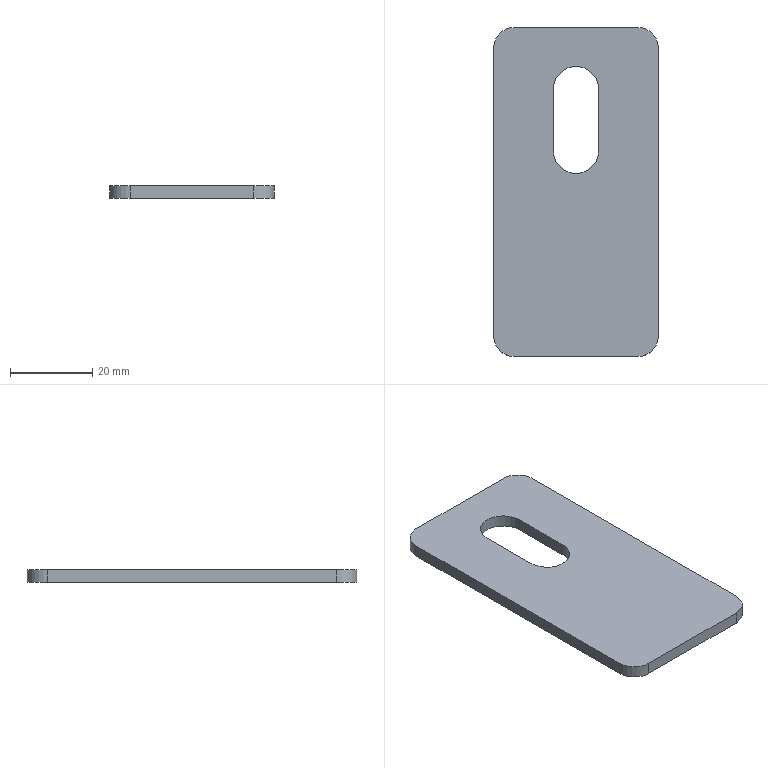Part | STEP file | Part4 | 1 solid | 14 faces | box 40 x 80 x 3 mm | volume 8756 mm3 | plane 8 | cylinder 6 | commonest cylinder face diameters 10 x4 11 x2
STEP:
#1=CARTESIAN_POINT('',(0.,0.,0.));
#2=DIRECTION('',(0.,0.,1.));
#3=DIRECTION('',(1.,0.,0.));
#4=AXIS2_PLACEMENT_3D('',#1,#2,#3);
#5=CARTESIAN_POINT('',(25.5,-30.,0.));
#6=VERTEX_POINT('',#5);
#7=CARTESIAN_POINT('',(25.5,-15.,0.));
#8=VERTEX_POINT('',#7);
#9=CARTESIAN_POINT('',(25.5,-35.,0.));
#10=DIRECTION('',(0.,1.,0.));
#11=VECTOR('',#10,1.);
#12=LINE('',#9,#11);
#13=CARTESIAN_POINT('',(25.5,-30.,0.));
#14=DIRECTION('',(1.,0.,0.));
#15=DIRECTION('',(0.,1.,0.));
#16=AXIS2_PLACEMENT_3D('',#13,#14,#15);
#17=PLANE('',#16);
#18=CARTESIAN_POINT('',(-5.,0.));
#19=DIRECTION('',(1.,0.));
#20=VECTOR('',#19,1.);
#21=LINE('',#18,#20);
#22=(GEOMETRIC_REPRESENTATION_CONTEXT(2)PARAMETRIC_REPRESENTATION_CONTEXT()REPRESENTATION_CONTEXT('',''));
#23=DEFINITIONAL_REPRESENTATION('',(#21),#22);
#24=PCURVE('',#17,#23);
#25=CARTESIAN_POINT('',(20.,-40.,0.));
#26=DIRECTION('',(0.,0.,1.));
#27=DIRECTION('',(1.,0.,0.));
#28=AXIS2_PLACEMENT_3D('',#25,#26,#27);
#29=PLANE('',#28);
#30=CARTESIAN_POINT('',(5.5,5.));
#31=DIRECTION('',(0.,1.));
#32=VECTOR('',#31,1.);
#33=LINE('',#30,#32);
#34=(GEOMETRIC_REPRESENTATION_CONTEXT(2)PARAMETRIC_REPRESENTATION_CONTEXT()REPRESENTATION_CONTEXT('',''));
#35=DEFINITIONAL_REPRESENTATION('',(#33),#34);
#36=PCURVE('',#29,#35);
#37=SURFACE_CURVE('',#12,(#24,#36),.PCURVE_S1.);
#38=EDGE_CURVE('',#6,#8,#37,.T.);
#39=ORIENTED_EDGE('',*,*,#38,.F.);
#40=CARTESIAN_POINT('',(25.5,-30.,3.));
#41=VERTEX_POINT('',#40);
#42=CARTESIAN_POINT('',(25.5,-30.,0.));
#43=DIRECTION('',(0.,0.,-1.));
#44=VECTOR('',#43,1.);
#45=LINE('',#42,#44);
#46=CARTESIAN_POINT('',(0.,0.));
#47=DIRECTION('',(0.,-1.));
#48=VECTOR('',#47,1.);
#49=LINE('',#46,#48);
#50=(GEOMETRIC_REPRESENTATION_CONTEXT(2)PARAMETRIC_REPRESENTATION_CONTEXT()REPRESENTATION_CONTEXT('',''));
#51=DEFINITIONAL_REPRESENTATION('',(#49),#50);
#52=PCURVE('',#17,#51);
#53=CARTESIAN_POINT('',(20.,-30.,0.));
#54=DIRECTION('',(0.,0.,1.));
#55=DIRECTION('',(-1.,0.,0.));
#56=AXIS2_PLACEMENT_3D('',#53,#54,#55);
#57=CYLINDRICAL_SURFACE('',#56,5.5);
#58=CARTESIAN_POINT('',(3.142,0.));
#59=DIRECTION('',(0.,-1.));
#60=VECTOR('',#59,1.);
#61=LINE('',#58,#60);
#62=(GEOMETRIC_REPRESENTATION_CONTEXT(2)PARAMETRIC_REPRESENTATION_CONTEXT()REPRESENTATION_CONTEXT('',''));
#63=DEFINITIONAL_REPRESENTATION('',(#61),#62);
#64=PCURVE('',#57,#63);
#65=SURFACE_CURVE('',#45,(#52,#64),.PCURVE_S1.);
#66=EDGE_CURVE('',#41,#6,#65,.T.);
#67=ORIENTED_EDGE('',*,*,#66,.F.);
#68=CARTESIAN_POINT('',(25.5,-15.,3.));
#69=VERTEX_POINT('',#68);
#70=CARTESIAN_POINT('',(25.5,-35.,3.));
#71=DIRECTION('',(0.,-1.,0.));
#72=VECTOR('',#71,1.);
#73=LINE('',#70,#72);
#74=CARTESIAN_POINT('',(-5.,3.));
#75=DIRECTION('',(-1.,0.));
#76=VECTOR('',#75,1.);
#77=LINE('',#74,#76);
#78=(GEOMETRIC_REPRESENTATION_CONTEXT(2)PARAMETRIC_REPRESENTATION_CONTEXT()REPRESENTATION_CONTEXT('',''));
#79=DEFINITIONAL_REPRESENTATION('',(#77),#78);
#80=PCURVE('',#17,#79);
#81=CARTESIAN_POINT('',(20.,-40.,3.));
#82=DIRECTION('',(0.,0.,1.));
#83=DIRECTION('',(1.,0.,0.));
#84=AXIS2_PLACEMENT_3D('',#81,#82,#83);
#85=PLANE('',#84);
#86=CARTESIAN_POINT('',(5.5,5.));
#87=DIRECTION('',(0.,-1.));
#88=VECTOR('',#87,1.);
#89=LINE('',#86,#88);
#90=(GEOMETRIC_REPRESENTATION_CONTEXT(2)PARAMETRIC_REPRESENTATION_CONTEXT()REPRESENTATION_CONTEXT('',''));
#91=DEFINITIONAL_REPRESENTATION('',(#89),#90);
#92=PCURVE('',#85,#91);
#93=SURFACE_CURVE('',#73,(#80,#92),.PCURVE_S1.);
#94=EDGE_CURVE('',#69,#41,#93,.T.);
#95=ORIENTED_EDGE('',*,*,#94,.F.);
#96=CARTESIAN_POINT('',(25.5,-15.,0.));
#97=DIRECTION('',(0.,0.,-1.));
#98=VECTOR('',#97,1.);
#99=LINE('',#96,#98);
#100=CARTESIAN_POINT('',(15.,0.));
#101=DIRECTION('',(0.,-1.));
#102=VECTOR('',#101,1.);
#103=LINE('',#100,#102);
#104=(GEOMETRIC_REPRESENTATION_CONTEXT(2)PARAMETRIC_REPRESENTATION_CONTEXT()REPRESENTATION_CONTEXT('',''));
#105=DEFINITIONAL_REPRESENTATION('',(#103),#104);
#106=PCURVE('',#17,#105);
#107=CARTESIAN_POINT('',(20.,-15.,0.));
#108=DIRECTION('',(0.,0.,1.));
#109=DIRECTION('',(-1.,0.,0.));
#110=AXIS2_PLACEMENT_3D('',#107,#108,#109);
#111=CYLINDRICAL_SURFACE('',#110,5.5);
#112=CARTESIAN_POINT('',(3.142,0.));
#113=DIRECTION('',(0.,-1.));
#114=VECTOR('',#113,1.);
#115=LINE('',#112,#114);
#116=(GEOMETRIC_REPRESENTATION_CONTEXT(2)PARAMETRIC_REPRESENTATION_CONTEXT()REPRESENTATION_CONTEXT('',''));
#117=DEFINITIONAL_REPRESENTATION('',(#115),#116);
#118=PCURVE('',#111,#117);
#119=SURFACE_CURVE('',#99,(#106,#118),.PCURVE_S1.);
#120=EDGE_CURVE('',#69,#8,#119,.T.);
#121=ORIENTED_EDGE('',*,*,#120,.T.);
#122=EDGE_LOOP('',(#39,#67,#95,#121));
#123=FACE_BOUND('',#122,.T.);
#124=ADVANCED_FACE('',(#123),#17,.F.);
#125=CARTESIAN_POINT('',(14.5,-15.,0.));
#126=VERTEX_POINT('',#125);
#127=CARTESIAN_POINT('',(14.5,-30.,0.));
#128=VERTEX_POINT('',#127);
#129=CARTESIAN_POINT('',(14.5,-27.5,0.));
#130=DIRECTION('',(0.,-1.,0.));
#131=VECTOR('',#130,1.);
#132=LINE('',#129,#131);
#133=CARTESIAN_POINT('',(14.5,-15.,0.));
#134=DIRECTION('',(-1.,0.,0.));
#135=DIRECTION('',(0.,-1.,0.));
#136=AXIS2_PLACEMENT_3D('',#133,#134,#135);
#137=PLANE('',#136);
#138=CARTESIAN_POINT('',(12.5,0.));
#139=DIRECTION('',(1.,0.));
#140=VECTOR('',#139,1.);
#141=LINE('',#138,#140);
#142=(GEOMETRIC_REPRESENTATION_CONTEXT(2)PARAMETRIC_REPRESENTATION_CONTEXT()REPRESENTATION_CONTEXT('',''));
#143=DEFINITIONAL_REPRESENTATION('',(#141),#142);
#144=PCURVE('',#137,#143);
#145=CARTESIAN_POINT('',(-5.5,12.5));
#146=DIRECTION('',(0.,-1.));
#147=VECTOR('',#146,1.);
#148=LINE('',#145,#147);
#149=(GEOMETRIC_REPRESENTATION_CONTEXT(2)PARAMETRIC_REPRESENTATION_CONTEXT()REPRESENTATION_CONTEXT('',''));
#150=DEFINITIONAL_REPRESENTATION('',(#148),#149);
#151=PCURVE('',#29,#150);
#152=SURFACE_CURVE('',#132,(#144,#151),.PCURVE_S1.);
#153=EDGE_CURVE('',#126,#128,#152,.T.);
#154=ORIENTED_EDGE('',*,*,#153,.F.);
#155=CARTESIAN_POINT('',(14.5,-15.,3.));
#156=VERTEX_POINT('',#155);
#157=CARTESIAN_POINT('',(14.5,-15.,0.));
#158=DIRECTION('',(0.,0.,-1.));
#159=VECTOR('',#158,1.);
#160=LINE('',#157,#159);
#161=CARTESIAN_POINT('',(0.,0.));
#162=DIRECTION('',(0.,-1.));
#163=VECTOR('',#162,1.);
#164=LINE('',#161,#163);
#165=(GEOMETRIC_REPRESENTATION_CONTEXT(2)PARAMETRIC_REPRESENTATION_CONTEXT()REPRESENTATION_CONTEXT('',''));
#166=DEFINITIONAL_REPRESENTATION('',(#164),#165);
#167=PCURVE('',#137,#166);
#168=CARTESIAN_POINT('',(6.283,0.));
#169=DIRECTION('',(0.,-1.));
#170=VECTOR('',#169,1.);
#171=LINE('',#168,#170);
#172=(GEOMETRIC_REPRESENTATION_CONTEXT(2)PARAMETRIC_REPRESENTATION_CONTEXT()REPRESENTATION_CONTEXT('',''));
#173=DEFINITIONAL_REPRESENTATION('',(#171),#172);
#174=PCURVE('',#111,#173);
#175=SURFACE_CURVE('',#160,(#167,#174),.PCURVE_S1.);
#176=EDGE_CURVE('',#156,#126,#175,.T.);
#177=ORIENTED_EDGE('',*,*,#176,.F.);
#178=CARTESIAN_POINT('',(14.5,-30.,3.));
#179=VERTEX_POINT('',#178);
#180=CARTESIAN_POINT('',(14.5,-27.5,3.));
#181=DIRECTION('',(0.,1.,0.));
#182=VECTOR('',#181,1.);
#183=LINE('',#180,#182);
#184=CARTESIAN_POINT('',(12.5,3.));
#185=DIRECTION('',(-1.,0.));
#186=VECTOR('',#185,1.);
#187=LINE('',#184,#186);
#188=(GEOMETRIC_REPRESENTATION_CONTEXT(2)PARAMETRIC_REPRESENTATION_CONTEXT()REPRESENTATION_CONTEXT('',''));
#189=DEFINITIONAL_REPRESENTATION('',(#187),#188);
#190=PCURVE('',#137,#189);
#191=CARTESIAN_POINT('',(-5.5,12.5));
#192=DIRECTION('',(0.,1.));
#193=VECTOR('',#192,1.);
#194=LINE('',#191,#193);
#195=(GEOMETRIC_REPRESENTATION_CONTEXT(2)PARAMETRIC_REPRESENTATION_CONTEXT()REPRESENTATION_CONTEXT('',''));
#196=DEFINITIONAL_REPRESENTATION('',(#194),#195);
#197=PCURVE('',#85,#196);
#198=SURFACE_CURVE('',#183,(#190,#197),.PCURVE_S1.);
#199=EDGE_CURVE('',#179,#156,#198,.T.);
#200=ORIENTED_EDGE('',*,*,#199,.F.);
#201=CARTESIAN_POINT('',(14.5,-30.,0.));
#202=DIRECTION('',(0.,0.,1.));
#203=VECTOR('',#202,1.);
#204=LINE('',#201,#203);
#205=CARTESIAN_POINT('',(15.,0.));
#206=DIRECTION('',(0.,1.));
#207=VECTOR('',#206,1.);
#208=LINE('',#205,#207);
#209=(GEOMETRIC_REPRESENTATION_CONTEXT(2)PARAMETRIC_REPRESENTATION_CONTEXT()REPRESENTATION_CONTEXT('',''));
#210=DEFINITIONAL_REPRESENTATION('',(#208),#209);
#211=PCURVE('',#137,#210);
#212=CARTESIAN_POINT('',(0.,0.));
#213=DIRECTION('',(0.,1.));
#214=VECTOR('',#213,1.);
#215=LINE('',#212,#214);
#216=(GEOMETRIC_REPRESENTATION_CONTEXT(2)PARAMETRIC_REPRESENTATION_CONTEXT()REPRESENTATION_CONTEXT('',''));
#217=DEFINITIONAL_REPRESENTATION('',(#215),#216);
#218=PCURVE('',#57,#217);
#219=SURFACE_CURVE('',#204,(#211,#218),.PCURVE_S1.);
#220=EDGE_CURVE('',#128,#179,#219,.T.);
#221=ORIENTED_EDGE('',*,*,#220,.F.);
#222=EDGE_LOOP('',(#154,#177,#200,#221));
#223=FACE_BOUND('',#222,.T.);
#224=ADVANCED_FACE('',(#223),#137,.F.);
#225=CARTESIAN_POINT('',(0.,-5.,0.));
#226=VERTEX_POINT('',#225);
#227=CARTESIAN_POINT('',(0.,-75.,0.));
#228=VERTEX_POINT('',#227);
#229=CARTESIAN_POINT('',(0.,-5.,0.));
#230=DIRECTION('',(0.,-1.,0.));
#231=VECTOR('',#230,1.);
#232=LINE('',#229,#231);
#233=CARTESIAN_POINT('',(-20.,35.));
#234=DIRECTION('',(0.,-1.));
#235=VECTOR('',#234,1.);
#236=LINE('',#233,#235);
#237=(GEOMETRIC_REPRESENTATION_CONTEXT(2)PARAMETRIC_REPRESENTATION_CONTEXT()REPRESENTATION_CONTEXT('',''));
#238=DEFINITIONAL_REPRESENTATION('',(#236),#237);
#239=PCURVE('',#29,#238);
#240=CARTESIAN_POINT('',(0.,-5.,0.));
#241=DIRECTION('',(-1.,0.,0.));
#242=DIRECTION('',(0.,-1.,0.));
#243=AXIS2_PLACEMENT_3D('',#240,#241,#242);
#244=PLANE('',#243);
#245=CARTESIAN_POINT('',(0.,0.));
#246=DIRECTION('',(1.,0.));
#247=VECTOR('',#246,1.);
#248=LINE('',#245,#247);
#249=(GEOMETRIC_REPRESENTATION_CONTEXT(2)PARAMETRIC_REPRESENTATION_CONTEXT()REPRESENTATION_CONTEXT('',''));
#250=DEFINITIONAL_REPRESENTATION('',(#248),#249);
#251=PCURVE('',#244,#250);
#252=SURFACE_CURVE('',#232,(#239,#251),.PCURVE_S1.);
#253=EDGE_CURVE('',#226,#228,#252,.T.);
#254=ORIENTED_EDGE('',*,*,#253,.F.);
#255=CARTESIAN_POINT('',(5.,0.,0.));
#256=VERTEX_POINT('',#255);
#257=CARTESIAN_POINT('',(5.,-5.,0.));
#258=DIRECTION('',(0.,0.,1.));
#259=DIRECTION('',(0.,1.,0.));
#260=AXIS2_PLACEMENT_3D('',#257,#258,#259);
#261=CIRCLE('',#260,5.);
#262=CARTESIAN_POINT('',(-15.,35.));
#263=DIRECTION('',(0.,1.));
#264=AXIS2_PLACEMENT_2D('',#262,#263);
#265=CIRCLE('',#264,5.);
#266=(GEOMETRIC_REPRESENTATION_CONTEXT(2)PARAMETRIC_REPRESENTATION_CONTEXT()REPRESENTATION_CONTEXT('',''));
#267=DEFINITIONAL_REPRESENTATION('',(#265),#266);
#268=PCURVE('',#29,#267);
#269=CARTESIAN_POINT('',(5.,-5.,0.));
#270=DIRECTION('',(0.,0.,1.));
#271=DIRECTION('',(0.,1.,0.));
#272=AXIS2_PLACEMENT_3D('',#269,#270,#271);
#273=CYLINDRICAL_SURFACE('',#272,5.);
#274=CARTESIAN_POINT('',(0.,0.));
#275=DIRECTION('',(1.,0.));
#276=VECTOR('',#275,1.);
#277=LINE('',#274,#276);
#278=(GEOMETRIC_REPRESENTATION_CONTEXT(2)PARAMETRIC_REPRESENTATION_CONTEXT()REPRESENTATION_CONTEXT('',''));
#279=DEFINITIONAL_REPRESENTATION('',(#277),#278);
#280=PCURVE('',#273,#279);
#281=SURFACE_CURVE('',#261,(#268,#280),.PCURVE_S1.);
#282=EDGE_CURVE('',#256,#226,#281,.T.);
#283=ORIENTED_EDGE('',*,*,#282,.F.);
#284=CARTESIAN_POINT('',(35.,0.,0.));
#285=VERTEX_POINT('',#284);
#286=CARTESIAN_POINT('',(35.,0.,0.));
#287=DIRECTION('',(-1.,0.,0.));
#288=VECTOR('',#287,1.);
#289=LINE('',#286,#288);
#290=CARTESIAN_POINT('',(15.,40.));
#291=DIRECTION('',(-1.,0.));
#292=VECTOR('',#291,1.);
#293=LINE('',#290,#292);
#294=(GEOMETRIC_REPRESENTATION_CONTEXT(2)PARAMETRIC_REPRESENTATION_CONTEXT()REPRESENTATION_CONTEXT('',''));
#295=DEFINITIONAL_REPRESENTATION('',(#293),#294);
#296=PCURVE('',#29,#295);
#297=CARTESIAN_POINT('',(35.,0.,0.));
#298=DIRECTION('',(0.,1.,0.));
#299=DIRECTION('',(-1.,0.,0.));
#300=AXIS2_PLACEMENT_3D('',#297,#298,#299);
#301=PLANE('',#300);
#302=CARTESIAN_POINT('',(0.,0.));
#303=DIRECTION('',(1.,0.));
#304=VECTOR('',#303,1.);
#305=LINE('',#302,#304);
#306=(GEOMETRIC_REPRESENTATION_CONTEXT(2)PARAMETRIC_REPRESENTATION_CONTEXT()REPRESENTATION_CONTEXT('',''));
#307=DEFINITIONAL_REPRESENTATION('',(#305),#306);
#308=PCURVE('',#301,#307);
#309=SURFACE_CURVE('',#289,(#296,#308),.PCURVE_S1.);
#310=EDGE_CURVE('',#285,#256,#309,.T.);
#311=ORIENTED_EDGE('',*,*,#310,.F.);
#312=CARTESIAN_POINT('',(40.,-5.,0.));
#313=VERTEX_POINT('',#312);
#314=CARTESIAN_POINT('',(35.,-5.,0.));
#315=DIRECTION('',(0.,0.,1.));
#316=DIRECTION('',(1.,0.,0.));
#317=AXIS2_PLACEMENT_3D('',#314,#315,#316);
#318=CIRCLE('',#317,5.);
#319=CARTESIAN_POINT('',(15.,35.));
#320=DIRECTION('',(1.,0.));
#321=AXIS2_PLACEMENT_2D('',#319,#320);
#322=CIRCLE('',#321,5.);
#323=(GEOMETRIC_REPRESENTATION_CONTEXT(2)PARAMETRIC_REPRESENTATION_CONTEXT()REPRESENTATION_CONTEXT('',''));
#324=DEFINITIONAL_REPRESENTATION('',(#322),#323);
#325=PCURVE('',#29,#324);
#326=CARTESIAN_POINT('',(35.,-5.,0.));
#327=DIRECTION('',(0.,0.,1.));
#328=DIRECTION('',(1.,0.,0.));
#329=AXIS2_PLACEMENT_3D('',#326,#327,#328);
#330=CYLINDRICAL_SURFACE('',#329,5.);
#331=CARTESIAN_POINT('',(0.,0.));
#332=DIRECTION('',(1.,0.));
#333=VECTOR('',#332,1.);
#334=LINE('',#331,#333);
#335=(GEOMETRIC_REPRESENTATION_CONTEXT(2)PARAMETRIC_REPRESENTATION_CONTEXT()REPRESENTATION_CONTEXT('',''));
#336=DEFINITIONAL_REPRESENTATION('',(#334),#335);
#337=PCURVE('',#330,#336);
#338=SURFACE_CURVE('',#318,(#325,#337),.PCURVE_S1.);
#339=EDGE_CURVE('',#313,#285,#338,.T.);
#340=ORIENTED_EDGE('',*,*,#339,.F.);
#341=CARTESIAN_POINT('',(40.,-75.,0.));
#342=VERTEX_POINT('',#341);
#343=CARTESIAN_POINT('',(40.,-75.,0.));
#344=DIRECTION('',(0.,1.,0.));
#345=VECTOR('',#344,1.);
#346=LINE('',#343,#345);
#347=CARTESIAN_POINT('',(20.,-35.));
#348=DIRECTION('',(0.,1.));
#349=VECTOR('',#348,1.);
#350=LINE('',#347,#349);
#351=(GEOMETRIC_REPRESENTATION_CONTEXT(2)PARAMETRIC_REPRESENTATION_CONTEXT()REPRESENTATION_CONTEXT('',''));
#352=DEFINITIONAL_REPRESENTATION('',(#350),#351);
#353=PCURVE('',#29,#352);
#354=CARTESIAN_POINT('',(40.,-75.,0.));
#355=DIRECTION('',(1.,0.,0.));
#356=DIRECTION('',(0.,1.,0.));
#357=AXIS2_PLACEMENT_3D('',#354,#355,#356);
#358=PLANE('',#357);
#359=CARTESIAN_POINT('',(0.,0.));
#360=DIRECTION('',(1.,0.));
#361=VECTOR('',#360,1.);
#362=LINE('',#359,#361);
#363=(GEOMETRIC_REPRESENTATION_CONTEXT(2)PARAMETRIC_REPRESENTATION_CONTEXT()REPRESENTATION_CONTEXT('',''));
#364=DEFINITIONAL_REPRESENTATION('',(#362),#363);
#365=PCURVE('',#358,#364);
#366=SURFACE_CURVE('',#346,(#353,#365),.PCURVE_S1.);
#367=EDGE_CURVE('',#342,#313,#366,.T.);
#368=ORIENTED_EDGE('',*,*,#367,.F.);
#369=CARTESIAN_POINT('',(35.,-80.,0.));
#370=VERTEX_POINT('',#369);
#371=CARTESIAN_POINT('',(35.,-75.,0.));
#372=DIRECTION('',(0.,0.,1.));
#373=DIRECTION('',(0.,-1.,0.));
#374=AXIS2_PLACEMENT_3D('',#371,#372,#373);
#375=CIRCLE('',#374,5.);
#376=CARTESIAN_POINT('',(15.,-35.));
#377=DIRECTION('',(0.,-1.));
#378=AXIS2_PLACEMENT_2D('',#376,#377);
#379=CIRCLE('',#378,5.);
#380=(GEOMETRIC_REPRESENTATION_CONTEXT(2)PARAMETRIC_REPRESENTATION_CONTEXT()REPRESENTATION_CONTEXT('',''));
#381=DEFINITIONAL_REPRESENTATION('',(#379),#380);
#382=PCURVE('',#29,#381);
#383=CARTESIAN_POINT('',(35.,-75.,0.));
#384=DIRECTION('',(0.,0.,1.));
#385=DIRECTION('',(0.,-1.,0.));
#386=AXIS2_PLACEMENT_3D('',#383,#384,#385);
#387=CYLINDRICAL_SURFACE('',#386,5.);
#388=CARTESIAN_POINT('',(0.,0.));
#389=DIRECTION('',(1.,0.));
#390=VECTOR('',#389,1.);
#391=LINE('',#388,#390);
#392=(GEOMETRIC_REPRESENTATION_CONTEXT(2)PARAMETRIC_REPRESENTATION_CONTEXT()REPRESENTATION_CONTEXT('',''));
#393=DEFINITIONAL_REPRESENTATION('',(#391),#392);
#394=PCURVE('',#387,#393);
#395=SURFACE_CURVE('',#375,(#382,#394),.PCURVE_S1.);
#396=EDGE_CURVE('',#370,#342,#395,.T.);
#397=ORIENTED_EDGE('',*,*,#396,.F.);
#398=CARTESIAN_POINT('',(5.,-80.,0.));
#399=VERTEX_POINT('',#398);
#400=CARTESIAN_POINT('',(5.,-80.,0.));
#401=DIRECTION('',(1.,0.,0.));
#402=VECTOR('',#401,1.);
#403=LINE('',#400,#402);
#404=CARTESIAN_POINT('',(-15.,-40.));
#405=DIRECTION('',(1.,0.));
#406=VECTOR('',#405,1.);
#407=LINE('',#404,#406);
#408=(GEOMETRIC_REPRESENTATION_CONTEXT(2)PARAMETRIC_REPRESENTATION_CONTEXT()REPRESENTATION_CONTEXT('',''));
#409=DEFINITIONAL_REPRESENTATION('',(#407),#408);
#410=PCURVE('',#29,#409);
#411=CARTESIAN_POINT('',(5.,-80.,0.));
#412=DIRECTION('',(0.,-1.,0.));
#413=DIRECTION('',(1.,0.,0.));
#414=AXIS2_PLACEMENT_3D('',#411,#412,#413);
#415=PLANE('',#414);
#416=CARTESIAN_POINT('',(0.,0.));
#417=DIRECTION('',(1.,0.));
#418=VECTOR('',#417,1.);
#419=LINE('',#416,#418);
#420=(GEOMETRIC_REPRESENTATION_CONTEXT(2)PARAMETRIC_REPRESENTATION_CONTEXT()REPRESENTATION_CONTEXT('',''));
#421=DEFINITIONAL_REPRESENTATION('',(#419),#420);
#422=PCURVE('',#415,#421);
#423=SURFACE_CURVE('',#403,(#410,#422),.PCURVE_S1.);
#424=EDGE_CURVE('',#399,#370,#423,.T.);
#425=ORIENTED_EDGE('',*,*,#424,.F.);
#426=CARTESIAN_POINT('',(5.,-75.,0.));
#427=DIRECTION('',(0.,0.,1.));
#428=DIRECTION('',(-1.,0.,0.));
#429=AXIS2_PLACEMENT_3D('',#426,#427,#428);
#430=CIRCLE('',#429,5.);
#431=CARTESIAN_POINT('',(-15.,-35.));
#432=DIRECTION('',(-1.,0.));
#433=AXIS2_PLACEMENT_2D('',#431,#432);
#434=CIRCLE('',#433,5.);
#435=(GEOMETRIC_REPRESENTATION_CONTEXT(2)PARAMETRIC_REPRESENTATION_CONTEXT()REPRESENTATION_CONTEXT('',''));
#436=DEFINITIONAL_REPRESENTATION('',(#434),#435);
#437=PCURVE('',#29,#436);
#438=CARTESIAN_POINT('',(5.,-75.,0.));
#439=DIRECTION('',(0.,0.,1.));
#440=DIRECTION('',(-1.,0.,0.));
#441=AXIS2_PLACEMENT_3D('',#438,#439,#440);
#442=CYLINDRICAL_SURFACE('',#441,5.);
#443=CARTESIAN_POINT('',(0.,0.));
#444=DIRECTION('',(1.,0.));
#445=VECTOR('',#444,1.);
#446=LINE('',#443,#445);
#447=(GEOMETRIC_REPRESENTATION_CONTEXT(2)PARAMETRIC_REPRESENTATION_CONTEXT()REPRESENTATION_CONTEXT('',''));
#448=DEFINITIONAL_REPRESENTATION('',(#446),#447);
#449=PCURVE('',#442,#448);
#450=SURFACE_CURVE('',#430,(#437,#449),.PCURVE_S1.);
#451=EDGE_CURVE('',#228,#399,#450,.T.);
#452=ORIENTED_EDGE('',*,*,#451,.F.);
#453=EDGE_LOOP('',(#254,#283,#311,#340,#368,#397,#425,#452));
#454=FACE_BOUND('',#453,.T.);
#455=ORIENTED_EDGE('',*,*,#38,.T.);
#456=CARTESIAN_POINT('',(20.,-15.,0.));
#457=DIRECTION('',(0.,0.,1.));
#458=DIRECTION('',(-1.,0.,0.));
#459=AXIS2_PLACEMENT_3D('',#456,#457,#458);
#460=CIRCLE('',#459,5.5);
#461=CARTESIAN_POINT('',(0.,25.));
#462=DIRECTION('',(-1.,0.));
#463=AXIS2_PLACEMENT_2D('',#461,#462);
#464=CIRCLE('',#463,5.5);
#465=(GEOMETRIC_REPRESENTATION_CONTEXT(2)PARAMETRIC_REPRESENTATION_CONTEXT()REPRESENTATION_CONTEXT('',''));
#466=DEFINITIONAL_REPRESENTATION('',(#464),#465);
#467=PCURVE('',#29,#466);
#468=CARTESIAN_POINT('',(0.,0.));
#469=DIRECTION('',(1.,0.));
#470=VECTOR('',#469,1.);
#471=LINE('',#468,#470);
#472=(GEOMETRIC_REPRESENTATION_CONTEXT(2)PARAMETRIC_REPRESENTATION_CONTEXT()REPRESENTATION_CONTEXT('',''));
#473=DEFINITIONAL_REPRESENTATION('',(#471),#472);
#474=PCURVE('',#111,#473);
#475=SURFACE_CURVE('',#460,(#467,#474),.PCURVE_S1.);
#476=EDGE_CURVE('',#8,#126,#475,.T.);
#477=ORIENTED_EDGE('',*,*,#476,.T.);
#478=ORIENTED_EDGE('',*,*,#153,.T.);
#479=CARTESIAN_POINT('',(20.,-30.,0.));
#480=DIRECTION('',(0.,0.,1.));
#481=DIRECTION('',(-1.,0.,0.));
#482=AXIS2_PLACEMENT_3D('',#479,#480,#481);
#483=CIRCLE('',#482,5.5);
#484=CARTESIAN_POINT('',(0.,10.));
#485=DIRECTION('',(-1.,0.));
#486=AXIS2_PLACEMENT_2D('',#484,#485);
#487=CIRCLE('',#486,5.5);
#488=(GEOMETRIC_REPRESENTATION_CONTEXT(2)PARAMETRIC_REPRESENTATION_CONTEXT()REPRESENTATION_CONTEXT('',''));
#489=DEFINITIONAL_REPRESENTATION('',(#487),#488);
#490=PCURVE('',#29,#489);
#491=CARTESIAN_POINT('',(0.,0.));
#492=DIRECTION('',(1.,0.));
#493=VECTOR('',#492,1.);
#494=LINE('',#491,#493);
#495=(GEOMETRIC_REPRESENTATION_CONTEXT(2)PARAMETRIC_REPRESENTATION_CONTEXT()REPRESENTATION_CONTEXT('',''));
#496=DEFINITIONAL_REPRESENTATION('',(#494),#495);
#497=PCURVE('',#57,#496);
#498=SURFACE_CURVE('',#483,(#490,#497),.PCURVE_S1.);
#499=EDGE_CURVE('',#128,#6,#498,.T.);
#500=ORIENTED_EDGE('',*,*,#499,.T.);
#501=EDGE_LOOP('',(#455,#477,#478,#500));
#502=FACE_BOUND('',#501,.T.);
#503=ADVANCED_FACE('',(#454,#502),#29,.F.);
#504=CARTESIAN_POINT('',(20.,-30.,3.));
#505=DIRECTION('',(0.,0.,-1.));
#506=DIRECTION('',(-1.,0.,0.));
#507=AXIS2_PLACEMENT_3D('',#504,#505,#506);
#508=CIRCLE('',#507,5.5);
#509=CARTESIAN_POINT('',(6.283,3.));
#510=DIRECTION('',(-1.,0.));
#511=VECTOR('',#510,1.);
#512=LINE('',#509,#511);
#513=(GEOMETRIC_REPRESENTATION_CONTEXT(2)PARAMETRIC_REPRESENTATION_CONTEXT()REPRESENTATION_CONTEXT('',''));
#514=DEFINITIONAL_REPRESENTATION('',(#512),#513);
#515=PCURVE('',#57,#514);
#516=CARTESIAN_POINT('',(-5.5,10.));
#517=CARTESIAN_POINT('',(-5.5,19.526));
#518=CARTESIAN_POINT('',(2.75,14.763));
#519=CARTESIAN_POINT('',(11.,10.));
#520=CARTESIAN_POINT('',(2.75,5.237));
#521=CARTESIAN_POINT('',(-5.5,0.4737));
#522=CARTESIAN_POINT('',(-5.5,10.));
#523=(BOUNDED_CURVE()B_SPLINE_CURVE(2,(#516,#517,#518,#519,#520,#521,#522),.UNSPECIFIED.,.T.,.F.)B_SPLINE_CURVE_WITH_KNOTS((1,2,2,2,2,1),(-2.094,0.,2.094,4.189,6.283,8.378),.UNSPECIFIED.)CURVE()GEOMETRIC_REPRESENTATION_ITEM()RATIONAL_B_SPLINE_CURVE((1.,0.5,1.,0.5,1.,0.5,1.))REPRESENTATION_ITEM(''));
#524=(GEOMETRIC_REPRESENTATION_CONTEXT(2)PARAMETRIC_REPRESENTATION_CONTEXT()REPRESENTATION_CONTEXT('',''));
#525=DEFINITIONAL_REPRESENTATION('',(#523),#524);
#526=PCURVE('',#85,#525);
#527=SURFACE_CURVE('',#508,(#515,#526),.PCURVE_S1.);
#528=EDGE_CURVE('',#41,#179,#527,.T.);
#529=ORIENTED_EDGE('',*,*,#528,.T.);
#530=ORIENTED_EDGE('',*,*,#220,.F.);
#531=ORIENTED_EDGE('',*,*,#499,.T.);
#532=ORIENTED_EDGE('',*,*,#66,.F.);
#533=EDGE_LOOP('',(#529,#530,#531,#532));
#534=FACE_BOUND('',#533,.F.);
#535=ADVANCED_FACE('',(#534),#57,.F.);
#536=ORIENTED_EDGE('',*,*,#476,.T.);
#537=ORIENTED_EDGE('',*,*,#176,.F.);
#538=CARTESIAN_POINT('',(20.,-15.,3.));
#539=DIRECTION('',(0.,0.,-1.));
#540=DIRECTION('',(-1.,0.,0.));
#541=AXIS2_PLACEMENT_3D('',#538,#539,#540);
#542=CIRCLE('',#541,5.5);
#543=CARTESIAN_POINT('',(6.283,3.));
#544=DIRECTION('',(-1.,0.));
#545=VECTOR('',#544,1.);
#546=LINE('',#543,#545);
#547=(GEOMETRIC_REPRESENTATION_CONTEXT(2)PARAMETRIC_REPRESENTATION_CONTEXT()REPRESENTATION_CONTEXT('',''));
#548=DEFINITIONAL_REPRESENTATION('',(#546),#547);
#549=PCURVE('',#111,#548);
#550=CARTESIAN_POINT('',(-5.5,25.));
#551=CARTESIAN_POINT('',(-5.5,34.526));
#552=CARTESIAN_POINT('',(2.75,29.763));
#553=CARTESIAN_POINT('',(11.,25.));
#554=CARTESIAN_POINT('',(2.75,20.237));
#555=CARTESIAN_POINT('',(-5.5,15.474));
#556=CARTESIAN_POINT('',(-5.5,25.));
#557=(BOUNDED_CURVE()B_SPLINE_CURVE(2,(#550,#551,#552,#553,#554,#555,#556),.UNSPECIFIED.,.T.,.F.)B_SPLINE_CURVE_WITH_KNOTS((1,2,2,2,2,1),(-2.094,0.,2.094,4.189,6.283,8.378),.UNSPECIFIED.)CURVE()GEOMETRIC_REPRESENTATION_ITEM()RATIONAL_B_SPLINE_CURVE((1.,0.5,1.,0.5,1.,0.5,1.))REPRESENTATION_ITEM(''));
#558=(GEOMETRIC_REPRESENTATION_CONTEXT(2)PARAMETRIC_REPRESENTATION_CONTEXT()REPRESENTATION_CONTEXT('',''));
#559=DEFINITIONAL_REPRESENTATION('',(#557),#558);
#560=PCURVE('',#85,#559);
#561=SURFACE_CURVE('',#542,(#549,#560),.PCURVE_S1.);
#562=EDGE_CURVE('',#156,#69,#561,.T.);
#563=ORIENTED_EDGE('',*,*,#562,.T.);
#564=ORIENTED_EDGE('',*,*,#120,.T.);
#565=EDGE_LOOP('',(#536,#537,#563,#564));
#566=FACE_BOUND('',#565,.F.);
#567=ADVANCED_FACE('',(#566),#111,.F.);
#568=ORIENTED_EDGE('',*,*,#282,.T.);
#569=CARTESIAN_POINT('',(0.,-5.,3.));
#570=VERTEX_POINT('',#569);
#571=CARTESIAN_POINT('',(0.,-5.,0.));
#572=DIRECTION('',(0.,0.,1.));
#573=VECTOR('',#572,1.);
#574=LINE('',#571,#573);
#575=CARTESIAN_POINT('',(1.571,0.));
#576=DIRECTION('',(0.,1.));
#577=VECTOR('',#576,1.);
#578=LINE('',#575,#577);
#579=(GEOMETRIC_REPRESENTATION_CONTEXT(2)PARAMETRIC_REPRESENTATION_CONTEXT()REPRESENTATION_CONTEXT('',''));
#580=DEFINITIONAL_REPRESENTATION('',(#578),#579);
#581=PCURVE('',#273,#580);
#582=CARTESIAN_POINT('',(0.,0.));
#583=DIRECTION('',(0.,1.));
#584=VECTOR('',#583,1.);
#585=LINE('',#582,#584);
#586=(GEOMETRIC_REPRESENTATION_CONTEXT(2)PARAMETRIC_REPRESENTATION_CONTEXT()REPRESENTATION_CONTEXT('',''));
#587=DEFINITIONAL_REPRESENTATION('',(#585),#586);
#588=PCURVE('',#244,#587);
#589=SURFACE_CURVE('',#574,(#581,#588),.PCURVE_S1.);
#590=EDGE_CURVE('',#226,#570,#589,.T.);
#591=ORIENTED_EDGE('',*,*,#590,.T.);
#592=CARTESIAN_POINT('',(5.,0.,3.));
#593=VERTEX_POINT('',#592);
#594=CARTESIAN_POINT('',(5.,-5.,3.));
#595=DIRECTION('',(0.,0.,1.));
#596=DIRECTION('',(0.,1.,0.));
#597=AXIS2_PLACEMENT_3D('',#594,#595,#596);
#598=CIRCLE('',#597,5.);
#599=CARTESIAN_POINT('',(0.,3.));
#600=DIRECTION('',(1.,0.));
#601=VECTOR('',#600,1.);
#602=LINE('',#599,#601);
#603=(GEOMETRIC_REPRESENTATION_CONTEXT(2)PARAMETRIC_REPRESENTATION_CONTEXT()REPRESENTATION_CONTEXT('',''));
#604=DEFINITIONAL_REPRESENTATION('',(#602),#603);
#605=PCURVE('',#273,#604);
#606=CARTESIAN_POINT('',(-15.,35.));
#607=DIRECTION('',(0.,1.));
#608=AXIS2_PLACEMENT_2D('',#606,#607);
#609=CIRCLE('',#608,5.);
#610=(GEOMETRIC_REPRESENTATION_CONTEXT(2)PARAMETRIC_REPRESENTATION_CONTEXT()REPRESENTATION_CONTEXT('',''));
#611=DEFINITIONAL_REPRESENTATION('',(#609),#610);
#612=PCURVE('',#85,#611);
#613=SURFACE_CURVE('',#598,(#605,#612),.PCURVE_S1.);
#614=EDGE_CURVE('',#593,#570,#613,.T.);
#615=ORIENTED_EDGE('',*,*,#614,.F.);
#616=CARTESIAN_POINT('',(5.,0.,0.));
#617=DIRECTION('',(0.,0.,1.));
#618=VECTOR('',#617,1.);
#619=LINE('',#616,#618);
#620=CARTESIAN_POINT('',(0.,0.));
#621=DIRECTION('',(0.,1.));
#622=VECTOR('',#621,1.);
#623=LINE('',#620,#622);
#624=(GEOMETRIC_REPRESENTATION_CONTEXT(2)PARAMETRIC_REPRESENTATION_CONTEXT()REPRESENTATION_CONTEXT('',''));
#625=DEFINITIONAL_REPRESENTATION('',(#623),#624);
#626=PCURVE('',#273,#625);
#627=CARTESIAN_POINT('',(30.,0.));
#628=DIRECTION('',(0.,1.));
#629=VECTOR('',#628,1.);
#630=LINE('',#627,#629);
#631=(GEOMETRIC_REPRESENTATION_CONTEXT(2)PARAMETRIC_REPRESENTATION_CONTEXT()REPRESENTATION_CONTEXT('',''));
#632=DEFINITIONAL_REPRESENTATION('',(#630),#631);
#633=PCURVE('',#301,#632);
#634=SURFACE_CURVE('',#619,(#626,#633),.PCURVE_S1.);
#635=EDGE_CURVE('',#256,#593,#634,.T.);
#636=ORIENTED_EDGE('',*,*,#635,.F.);
#637=EDGE_LOOP('',(#568,#591,#615,#636));
#638=FACE_BOUND('',#637,.T.);
#639=ADVANCED_FACE('',(#638),#273,.T.);
#640=ORIENTED_EDGE('',*,*,#310,.T.);
#641=ORIENTED_EDGE('',*,*,#635,.T.);
#642=CARTESIAN_POINT('',(35.,0.,3.));
#643=VERTEX_POINT('',#642);
#644=CARTESIAN_POINT('',(35.,0.,3.));
#645=DIRECTION('',(-1.,0.,0.));
#646=VECTOR('',#645,1.);
#647=LINE('',#644,#646);
#648=CARTESIAN_POINT('',(0.,3.));
#649=DIRECTION('',(1.,0.));
#650=VECTOR('',#649,1.);
#651=LINE('',#648,#650);
#652=(GEOMETRIC_REPRESENTATION_CONTEXT(2)PARAMETRIC_REPRESENTATION_CONTEXT()REPRESENTATION_CONTEXT('',''));
#653=DEFINITIONAL_REPRESENTATION('',(#651),#652);
#654=PCURVE('',#301,#653);
#655=CARTESIAN_POINT('',(15.,40.));
#656=DIRECTION('',(-1.,0.));
#657=VECTOR('',#656,1.);
#658=LINE('',#655,#657);
#659=(GEOMETRIC_REPRESENTATION_CONTEXT(2)PARAMETRIC_REPRESENTATION_CONTEXT()REPRESENTATION_CONTEXT('',''));
#660=DEFINITIONAL_REPRESENTATION('',(#658),#659);
#661=PCURVE('',#85,#660);
#662=SURFACE_CURVE('',#647,(#654,#661),.PCURVE_S1.);
#663=EDGE_CURVE('',#643,#593,#662,.T.);
#664=ORIENTED_EDGE('',*,*,#663,.F.);
#665=CARTESIAN_POINT('',(35.,0.,0.));
#666=DIRECTION('',(0.,0.,1.));
#667=VECTOR('',#666,1.);
#668=LINE('',#665,#667);
#669=CARTESIAN_POINT('',(0.,0.));
#670=DIRECTION('',(0.,1.));
#671=VECTOR('',#670,1.);
#672=LINE('',#669,#671);
#673=(GEOMETRIC_REPRESENTATION_CONTEXT(2)PARAMETRIC_REPRESENTATION_CONTEXT()REPRESENTATION_CONTEXT('',''));
#674=DEFINITIONAL_REPRESENTATION('',(#672),#673);
#675=PCURVE('',#301,#674);
#676=CARTESIAN_POINT('',(1.571,0.));
#677=DIRECTION('',(0.,1.));
#678=VECTOR('',#677,1.);
#679=LINE('',#676,#678);
#680=(GEOMETRIC_REPRESENTATION_CONTEXT(2)PARAMETRIC_REPRESENTATION_CONTEXT()REPRESENTATION_CONTEXT('',''));
#681=DEFINITIONAL_REPRESENTATION('',(#679),#680);
#682=PCURVE('',#330,#681);
#683=SURFACE_CURVE('',#668,(#675,#682),.PCURVE_S1.);
#684=EDGE_CURVE('',#285,#643,#683,.T.);
#685=ORIENTED_EDGE('',*,*,#684,.F.);
#686=EDGE_LOOP('',(#640,#641,#664,#685));
#687=FACE_BOUND('',#686,.T.);
#688=ADVANCED_FACE('',(#687),#301,.T.);
#689=ORIENTED_EDGE('',*,*,#339,.T.);
#690=ORIENTED_EDGE('',*,*,#684,.T.);
#691=CARTESIAN_POINT('',(40.,-5.,3.));
#692=VERTEX_POINT('',#691);
#693=CARTESIAN_POINT('',(35.,-5.,3.));
#694=DIRECTION('',(0.,0.,1.));
#695=DIRECTION('',(1.,0.,0.));
#696=AXIS2_PLACEMENT_3D('',#693,#694,#695);
#697=CIRCLE('',#696,5.);
#698=CARTESIAN_POINT('',(0.,3.));
#699=DIRECTION('',(1.,0.));
#700=VECTOR('',#699,1.);
#701=LINE('',#698,#700);
#702=(GEOMETRIC_REPRESENTATION_CONTEXT(2)PARAMETRIC_REPRESENTATION_CONTEXT()REPRESENTATION_CONTEXT('',''));
#703=DEFINITIONAL_REPRESENTATION('',(#701),#702);
#704=PCURVE('',#330,#703);
#705=CARTESIAN_POINT('',(15.,35.));
#706=DIRECTION('',(1.,0.));
#707=AXIS2_PLACEMENT_2D('',#705,#706);
#708=CIRCLE('',#707,5.);
#709=(GEOMETRIC_REPRESENTATION_CONTEXT(2)PARAMETRIC_REPRESENTATION_CONTEXT()REPRESENTATION_CONTEXT('',''));
#710=DEFINITIONAL_REPRESENTATION('',(#708),#709);
#711=PCURVE('',#85,#710);
#712=SURFACE_CURVE('',#697,(#704,#711),.PCURVE_S1.);
#713=EDGE_CURVE('',#692,#643,#712,.T.);
#714=ORIENTED_EDGE('',*,*,#713,.F.);
#715=CARTESIAN_POINT('',(40.,-5.,0.));
#716=DIRECTION('',(0.,0.,1.));
#717=VECTOR('',#716,1.);
#718=LINE('',#715,#717);
#719=CARTESIAN_POINT('',(0.,0.));
#720=DIRECTION('',(0.,1.));
#721=VECTOR('',#720,1.);
#722=LINE('',#719,#721);
#723=(GEOMETRIC_REPRESENTATION_CONTEXT(2)PARAMETRIC_REPRESENTATION_CONTEXT()REPRESENTATION_CONTEXT('',''));
#724=DEFINITIONAL_REPRESENTATION('',(#722),#723);
#725=PCURVE('',#330,#724);
#726=CARTESIAN_POINT('',(70.,0.));
#727=DIRECTION('',(0.,1.));
#728=VECTOR('',#727,1.);
#729=LINE('',#726,#728);
#730=(GEOMETRIC_REPRESENTATION_CONTEXT(2)PARAMETRIC_REPRESENTATION_CONTEXT()REPRESENTATION_CONTEXT('',''));
#731=DEFINITIONAL_REPRESENTATION('',(#729),#730);
#732=PCURVE('',#358,#731);
#733=SURFACE_CURVE('',#718,(#725,#732),.PCURVE_S1.);
#734=EDGE_CURVE('',#313,#692,#733,.T.);
#735=ORIENTED_EDGE('',*,*,#734,.F.);
#736=EDGE_LOOP('',(#689,#690,#714,#735));
#737=FACE_BOUND('',#736,.T.);
#738=ADVANCED_FACE('',(#737),#330,.T.);
#739=ORIENTED_EDGE('',*,*,#367,.T.);
#740=ORIENTED_EDGE('',*,*,#734,.T.);
#741=CARTESIAN_POINT('',(40.,-75.,3.));
#742=VERTEX_POINT('',#741);
#743=CARTESIAN_POINT('',(40.,-75.,3.));
#744=DIRECTION('',(0.,1.,0.));
#745=VECTOR('',#744,1.);
#746=LINE('',#743,#745);
#747=CARTESIAN_POINT('',(0.,3.));
#748=DIRECTION('',(1.,0.));
#749=VECTOR('',#748,1.);
#750=LINE('',#747,#749);
#751=(GEOMETRIC_REPRESENTATION_CONTEXT(2)PARAMETRIC_REPRESENTATION_CONTEXT()REPRESENTATION_CONTEXT('',''));
#752=DEFINITIONAL_REPRESENTATION('',(#750),#751);
#753=PCURVE('',#358,#752);
#754=CARTESIAN_POINT('',(20.,-35.));
#755=DIRECTION('',(0.,1.));
#756=VECTOR('',#755,1.);
#757=LINE('',#754,#756);
#758=(GEOMETRIC_REPRESENTATION_CONTEXT(2)PARAMETRIC_REPRESENTATION_CONTEXT()REPRESENTATION_CONTEXT('',''));
#759=DEFINITIONAL_REPRESENTATION('',(#757),#758);
#760=PCURVE('',#85,#759);
#761=SURFACE_CURVE('',#746,(#753,#760),.PCURVE_S1.);
#762=EDGE_CURVE('',#742,#692,#761,.T.);
#763=ORIENTED_EDGE('',*,*,#762,.F.);
#764=CARTESIAN_POINT('',(40.,-75.,0.));
#765=DIRECTION('',(0.,0.,1.));
#766=VECTOR('',#765,1.);
#767=LINE('',#764,#766);
#768=CARTESIAN_POINT('',(0.,0.));
#769=DIRECTION('',(0.,1.));
#770=VECTOR('',#769,1.);
#771=LINE('',#768,#770);
#772=(GEOMETRIC_REPRESENTATION_CONTEXT(2)PARAMETRIC_REPRESENTATION_CONTEXT()REPRESENTATION_CONTEXT('',''));
#773=DEFINITIONAL_REPRESENTATION('',(#771),#772);
#774=PCURVE('',#358,#773);
#775=CARTESIAN_POINT('',(1.571,0.));
#776=DIRECTION('',(0.,1.));
#777=VECTOR('',#776,1.);
#778=LINE('',#775,#777);
#779=(GEOMETRIC_REPRESENTATION_CONTEXT(2)PARAMETRIC_REPRESENTATION_CONTEXT()REPRESENTATION_CONTEXT('',''));
#780=DEFINITIONAL_REPRESENTATION('',(#778),#779);
#781=PCURVE('',#387,#780);
#782=SURFACE_CURVE('',#767,(#774,#781),.PCURVE_S1.);
#783=EDGE_CURVE('',#342,#742,#782,.T.);
#784=ORIENTED_EDGE('',*,*,#783,.F.);
#785=EDGE_LOOP('',(#739,#740,#763,#784));
#786=FACE_BOUND('',#785,.T.);
#787=ADVANCED_FACE('',(#786),#358,.T.);
#788=ORIENTED_EDGE('',*,*,#396,.T.);
#789=ORIENTED_EDGE('',*,*,#783,.T.);
#790=CARTESIAN_POINT('',(35.,-80.,3.));
#791=VERTEX_POINT('',#790);
#792=CARTESIAN_POINT('',(35.,-75.,3.));
#793=DIRECTION('',(0.,0.,1.));
#794=DIRECTION('',(0.,-1.,0.));
#795=AXIS2_PLACEMENT_3D('',#792,#793,#794);
#796=CIRCLE('',#795,5.);
#797=CARTESIAN_POINT('',(0.,3.));
#798=DIRECTION('',(1.,0.));
#799=VECTOR('',#798,1.);
#800=LINE('',#797,#799);
#801=(GEOMETRIC_REPRESENTATION_CONTEXT(2)PARAMETRIC_REPRESENTATION_CONTEXT()REPRESENTATION_CONTEXT('',''));
#802=DEFINITIONAL_REPRESENTATION('',(#800),#801);
#803=PCURVE('',#387,#802);
#804=CARTESIAN_POINT('',(15.,-35.));
#805=DIRECTION('',(0.,-1.));
#806=AXIS2_PLACEMENT_2D('',#804,#805);
#807=CIRCLE('',#806,5.);
#808=(GEOMETRIC_REPRESENTATION_CONTEXT(2)PARAMETRIC_REPRESENTATION_CONTEXT()REPRESENTATION_CONTEXT('',''));
#809=DEFINITIONAL_REPRESENTATION('',(#807),#808);
#810=PCURVE('',#85,#809);
#811=SURFACE_CURVE('',#796,(#803,#810),.PCURVE_S1.);
#812=EDGE_CURVE('',#791,#742,#811,.T.);
#813=ORIENTED_EDGE('',*,*,#812,.F.);
#814=CARTESIAN_POINT('',(35.,-80.,0.));
#815=DIRECTION('',(0.,0.,1.));
#816=VECTOR('',#815,1.);
#817=LINE('',#814,#816);
#818=CARTESIAN_POINT('',(0.,0.));
#819=DIRECTION('',(0.,1.));
#820=VECTOR('',#819,1.);
#821=LINE('',#818,#820);
#822=(GEOMETRIC_REPRESENTATION_CONTEXT(2)PARAMETRIC_REPRESENTATION_CONTEXT()REPRESENTATION_CONTEXT('',''));
#823=DEFINITIONAL_REPRESENTATION('',(#821),#822);
#824=PCURVE('',#387,#823);
#825=CARTESIAN_POINT('',(30.,0.));
#826=DIRECTION('',(0.,1.));
#827=VECTOR('',#826,1.);
#828=LINE('',#825,#827);
#829=(GEOMETRIC_REPRESENTATION_CONTEXT(2)PARAMETRIC_REPRESENTATION_CONTEXT()REPRESENTATION_CONTEXT('',''));
#830=DEFINITIONAL_REPRESENTATION('',(#828),#829);
#831=PCURVE('',#415,#830);
#832=SURFACE_CURVE('',#817,(#824,#831),.PCURVE_S1.);
#833=EDGE_CURVE('',#370,#791,#832,.T.);
#834=ORIENTED_EDGE('',*,*,#833,.F.);
#835=EDGE_LOOP('',(#788,#789,#813,#834));
#836=FACE_BOUND('',#835,.T.);
#837=ADVANCED_FACE('',(#836),#387,.T.);
#838=ORIENTED_EDGE('',*,*,#424,.T.);
#839=ORIENTED_EDGE('',*,*,#833,.T.);
#840=CARTESIAN_POINT('',(5.,-80.,3.));
#841=VERTEX_POINT('',#840);
#842=CARTESIAN_POINT('',(5.,-80.,3.));
#843=DIRECTION('',(1.,0.,0.));
#844=VECTOR('',#843,1.);
#845=LINE('',#842,#844);
#846=CARTESIAN_POINT('',(0.,3.));
#847=DIRECTION('',(1.,0.));
#848=VECTOR('',#847,1.);
#849=LINE('',#846,#848);
#850=(GEOMETRIC_REPRESENTATION_CONTEXT(2)PARAMETRIC_REPRESENTATION_CONTEXT()REPRESENTATION_CONTEXT('',''));
#851=DEFINITIONAL_REPRESENTATION('',(#849),#850);
#852=PCURVE('',#415,#851);
#853=CARTESIAN_POINT('',(-15.,-40.));
#854=DIRECTION('',(1.,0.));
#855=VECTOR('',#854,1.);
#856=LINE('',#853,#855);
#857=(GEOMETRIC_REPRESENTATION_CONTEXT(2)PARAMETRIC_REPRESENTATION_CONTEXT()REPRESENTATION_CONTEXT('',''));
#858=DEFINITIONAL_REPRESENTATION('',(#856),#857);
#859=PCURVE('',#85,#858);
#860=SURFACE_CURVE('',#845,(#852,#859),.PCURVE_S1.);
#861=EDGE_CURVE('',#841,#791,#860,.T.);
#862=ORIENTED_EDGE('',*,*,#861,.F.);
#863=CARTESIAN_POINT('',(5.,-80.,0.));
#864=DIRECTION('',(0.,0.,1.));
#865=VECTOR('',#864,1.);
#866=LINE('',#863,#865);
#867=CARTESIAN_POINT('',(0.,0.));
#868=DIRECTION('',(0.,1.));
#869=VECTOR('',#868,1.);
#870=LINE('',#867,#869);
#871=(GEOMETRIC_REPRESENTATION_CONTEXT(2)PARAMETRIC_REPRESENTATION_CONTEXT()REPRESENTATION_CONTEXT('',''));
#872=DEFINITIONAL_REPRESENTATION('',(#870),#871);
#873=PCURVE('',#415,#872);
#874=CARTESIAN_POINT('',(1.571,0.));
#875=DIRECTION('',(0.,1.));
#876=VECTOR('',#875,1.);
#877=LINE('',#874,#876);
#878=(GEOMETRIC_REPRESENTATION_CONTEXT(2)PARAMETRIC_REPRESENTATION_CONTEXT()REPRESENTATION_CONTEXT('',''));
#879=DEFINITIONAL_REPRESENTATION('',(#877),#878);
#880=PCURVE('',#442,#879);
#881=SURFACE_CURVE('',#866,(#873,#880),.PCURVE_S1.);
#882=EDGE_CURVE('',#399,#841,#881,.T.);
#883=ORIENTED_EDGE('',*,*,#882,.F.);
#884=EDGE_LOOP('',(#838,#839,#862,#883));
#885=FACE_BOUND('',#884,.T.);
#886=ADVANCED_FACE('',(#885),#415,.T.);
#887=ORIENTED_EDGE('',*,*,#451,.T.);
#888=ORIENTED_EDGE('',*,*,#882,.T.);
#889=CARTESIAN_POINT('',(0.,-75.,3.));
#890=VERTEX_POINT('',#889);
#891=CARTESIAN_POINT('',(5.,-75.,3.));
#892=DIRECTION('',(0.,0.,1.));
#893=DIRECTION('',(-1.,0.,0.));
#894=AXIS2_PLACEMENT_3D('',#891,#892,#893);
#895=CIRCLE('',#894,5.);
#896=CARTESIAN_POINT('',(0.,3.));
#897=DIRECTION('',(1.,0.));
#898=VECTOR('',#897,1.);
#899=LINE('',#896,#898);
#900=(GEOMETRIC_REPRESENTATION_CONTEXT(2)PARAMETRIC_REPRESENTATION_CONTEXT()REPRESENTATION_CONTEXT('',''));
#901=DEFINITIONAL_REPRESENTATION('',(#899),#900);
#902=PCURVE('',#442,#901);
#903=CARTESIAN_POINT('',(-15.,-35.));
#904=DIRECTION('',(-1.,0.));
#905=AXIS2_PLACEMENT_2D('',#903,#904);
#906=CIRCLE('',#905,5.);
#907=(GEOMETRIC_REPRESENTATION_CONTEXT(2)PARAMETRIC_REPRESENTATION_CONTEXT()REPRESENTATION_CONTEXT('',''));
#908=DEFINITIONAL_REPRESENTATION('',(#906),#907);
#909=PCURVE('',#85,#908);
#910=SURFACE_CURVE('',#895,(#902,#909),.PCURVE_S1.);
#911=EDGE_CURVE('',#890,#841,#910,.T.);
#912=ORIENTED_EDGE('',*,*,#911,.F.);
#913=CARTESIAN_POINT('',(0.,-75.,0.));
#914=DIRECTION('',(0.,0.,1.));
#915=VECTOR('',#914,1.);
#916=LINE('',#913,#915);
#917=CARTESIAN_POINT('',(0.,0.));
#918=DIRECTION('',(0.,1.));
#919=VECTOR('',#918,1.);
#920=LINE('',#917,#919);
#921=(GEOMETRIC_REPRESENTATION_CONTEXT(2)PARAMETRIC_REPRESENTATION_CONTEXT()REPRESENTATION_CONTEXT('',''));
#922=DEFINITIONAL_REPRESENTATION('',(#920),#921);
#923=PCURVE('',#442,#922);
#924=CARTESIAN_POINT('',(70.,0.));
#925=DIRECTION('',(0.,1.));
#926=VECTOR('',#925,1.);
#927=LINE('',#924,#926);
#928=(GEOMETRIC_REPRESENTATION_CONTEXT(2)PARAMETRIC_REPRESENTATION_CONTEXT()REPRESENTATION_CONTEXT('',''));
#929=DEFINITIONAL_REPRESENTATION('',(#927),#928);
#930=PCURVE('',#244,#929);
#931=SURFACE_CURVE('',#916,(#923,#930),.PCURVE_S1.);
#932=EDGE_CURVE('',#228,#890,#931,.T.);
#933=ORIENTED_EDGE('',*,*,#932,.F.);
#934=EDGE_LOOP('',(#887,#888,#912,#933));
#935=FACE_BOUND('',#934,.T.);
#936=ADVANCED_FACE('',(#935),#442,.T.);
#937=ORIENTED_EDGE('',*,*,#253,.T.);
#938=ORIENTED_EDGE('',*,*,#932,.T.);
#939=CARTESIAN_POINT('',(0.,-5.,3.));
#940=DIRECTION('',(0.,-1.,0.));
#941=VECTOR('',#940,1.);
#942=LINE('',#939,#941);
#943=CARTESIAN_POINT('',(0.,3.));
#944=DIRECTION('',(1.,0.));
#945=VECTOR('',#944,1.);
#946=LINE('',#943,#945);
#947=(GEOMETRIC_REPRESENTATION_CONTEXT(2)PARAMETRIC_REPRESENTATION_CONTEXT()REPRESENTATION_CONTEXT('',''));
#948=DEFINITIONAL_REPRESENTATION('',(#946),#947);
#949=PCURVE('',#244,#948);
#950=CARTESIAN_POINT('',(-20.,35.));
#951=DIRECTION('',(0.,-1.));
#952=VECTOR('',#951,1.);
#953=LINE('',#950,#952);
#954=(GEOMETRIC_REPRESENTATION_CONTEXT(2)PARAMETRIC_REPRESENTATION_CONTEXT()REPRESENTATION_CONTEXT('',''));
#955=DEFINITIONAL_REPRESENTATION('',(#953),#954);
#956=PCURVE('',#85,#955);
#957=SURFACE_CURVE('',#942,(#949,#956),.PCURVE_S1.);
#958=EDGE_CURVE('',#570,#890,#957,.T.);
#959=ORIENTED_EDGE('',*,*,#958,.F.);
#960=ORIENTED_EDGE('',*,*,#590,.F.);
#961=EDGE_LOOP('',(#937,#938,#959,#960));
#962=FACE_BOUND('',#961,.T.);
#963=ADVANCED_FACE('',(#962),#244,.T.);
#964=ORIENTED_EDGE('',*,*,#958,.T.);
#965=ORIENTED_EDGE('',*,*,#911,.T.);
#966=ORIENTED_EDGE('',*,*,#861,.T.);
#967=ORIENTED_EDGE('',*,*,#812,.T.);
#968=ORIENTED_EDGE('',*,*,#762,.T.);
#969=ORIENTED_EDGE('',*,*,#713,.T.);
#970=ORIENTED_EDGE('',*,*,#663,.T.);
#971=ORIENTED_EDGE('',*,*,#614,.T.);
#972=EDGE_LOOP('',(#964,#965,#966,#967,#968,#969,#970,#971));
#973=FACE_BOUND('',#972,.T.);
#974=ORIENTED_EDGE('',*,*,#94,.T.);
#975=ORIENTED_EDGE('',*,*,#528,.T.);
#976=ORIENTED_EDGE('',*,*,#199,.T.);
#977=ORIENTED_EDGE('',*,*,#562,.T.);
#978=EDGE_LOOP('',(#974,#975,#976,#977));
#979=FACE_BOUND('',#978,.T.);
#980=ADVANCED_FACE('',(#973,#979),#85,.T.);
#981=CLOSED_SHELL('',(#124,#224,#503,#535,#567,#639,#688,#738,#787,#837,#886,#936,#963,#980));
#982=MANIFOLD_SOLID_BREP('',#981);
#983=(LENGTH_UNIT()NAMED_UNIT(*)SI_UNIT(.MILLI.,.METRE.));
#984=UNCERTAINTY_MEASURE_WITH_UNIT(LENGTH_MEASURE(0.0000001),#983,'','');
#985=(NAMED_UNIT(*)PLANE_ANGLE_UNIT()SI_UNIT($,.RADIAN.));
#986=(NAMED_UNIT(*)SI_UNIT($,.STERADIAN.)SOLID_ANGLE_UNIT());
#987=(GEOMETRIC_REPRESENTATION_CONTEXT(3)GLOBAL_UNCERTAINTY_ASSIGNED_CONTEXT((#984))GLOBAL_UNIT_ASSIGNED_CONTEXT((#983,#985,#986))REPRESENTATION_CONTEXT('',''));
#988=ADVANCED_BREP_SHAPE_REPRESENTATION('',(#4,#982),#987);